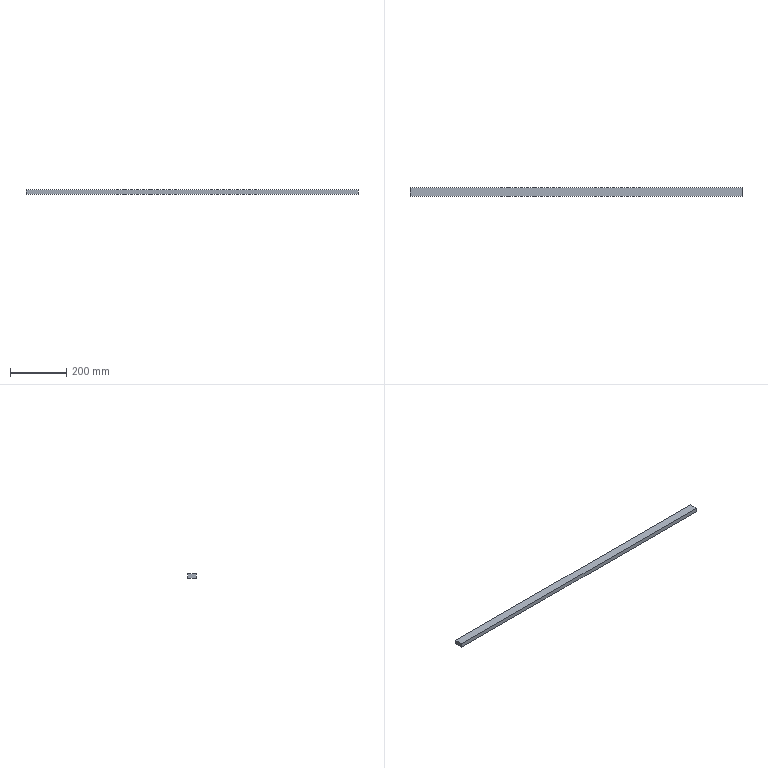Part | SolidWorks | features Extrusion 1 | 1 solid | 6 faces | box 1180 x 30 x 15 mm | volume 531000 mm3 | plane 6
STEP:
#1=CARTESIAN_POINT('',(590.,-15.,7.5));
#2=VERTEX_POINT('',#1);
#3=CARTESIAN_POINT('',(590.,-15.,-7.5));
#4=VERTEX_POINT('',#3);
#5=CARTESIAN_POINT('',(590.,-15.,7.5));
#6=DIRECTION('',(0.,0.,-1.));
#7=VECTOR('',#6,1000.);
#8=LINE('',#5,#7);
#9=EDGE_CURVE('',#2,#4,#8,.T.);
#10=ORIENTED_EDGE('',*,*,#9,.T.);
#11=CARTESIAN_POINT('',(590.,15.,-7.5));
#12=VERTEX_POINT('',#11);
#13=CARTESIAN_POINT('',(590.,15.,-7.5));
#14=DIRECTION('',(0.,-1.,0.));
#15=VECTOR('',#14,1000.);
#16=LINE('',#13,#15);
#17=EDGE_CURVE('',#12,#4,#16,.T.);
#18=ORIENTED_EDGE('',*,*,#17,.F.);
#19=CARTESIAN_POINT('',(590.,15.,7.5));
#20=VERTEX_POINT('',#19);
#21=CARTESIAN_POINT('',(590.,15.,7.5));
#22=DIRECTION('',(0.,0.,-1.));
#23=VECTOR('',#22,1000.);
#24=LINE('',#21,#23);
#25=EDGE_CURVE('',#20,#12,#24,.T.);
#26=ORIENTED_EDGE('',*,*,#25,.F.);
#27=CARTESIAN_POINT('',(590.,15.,7.5));
#28=DIRECTION('',(0.,-1.,0.));
#29=VECTOR('',#28,1000.);
#30=LINE('',#27,#29);
#31=EDGE_CURVE('',#20,#2,#30,.T.);
#32=ORIENTED_EDGE('',*,*,#31,.T.);
#33=EDGE_LOOP('',(#10,#18,#26,#32));
#34=FACE_OUTER_BOUND('',#33,.T.);
#35=CARTESIAN_POINT('',(590.,15.,7.5));
#36=DIRECTION('',(-1.,0.,0.));
#37=DIRECTION('',(0.,0.,1.));
#38=AXIS2_PLACEMENT_3D('',#35,#36,#37);
#39=PLANE('',#38);
#40=ADVANCED_FACE('',(#34),#39,.F.);
#41=CARTESIAN_POINT('',(-590.,-15.,-7.5));
#42=VERTEX_POINT('',#41);
#43=CARTESIAN_POINT('',(-590.,-15.,-7.5));
#44=DIRECTION('',(-1.,0.,0.));
#45=VECTOR('',#44,1000.);
#46=LINE('',#43,#45);
#47=EDGE_CURVE('',#4,#42,#46,.T.);
#48=ORIENTED_EDGE('',*,*,#47,.T.);
#49=CARTESIAN_POINT('',(-590.,15.,-7.5));
#50=VERTEX_POINT('',#49);
#51=CARTESIAN_POINT('',(-590.,15.,-7.5));
#52=DIRECTION('',(0.,-1.,0.));
#53=VECTOR('',#52,1000.);
#54=LINE('',#51,#53);
#55=EDGE_CURVE('',#50,#42,#54,.T.);
#56=ORIENTED_EDGE('',*,*,#55,.F.);
#57=CARTESIAN_POINT('',(-590.,15.,-7.5));
#58=DIRECTION('',(-1.,0.,0.));
#59=VECTOR('',#58,1000.);
#60=LINE('',#57,#59);
#61=EDGE_CURVE('',#12,#50,#60,.T.);
#62=ORIENTED_EDGE('',*,*,#61,.F.);
#63=ORIENTED_EDGE('',*,*,#17,.T.);
#64=EDGE_LOOP('',(#48,#56,#62,#63));
#65=FACE_OUTER_BOUND('',#64,.T.);
#66=CARTESIAN_POINT('',(-590.,15.,-7.5));
#67=DIRECTION('',(0.,0.,1.));
#68=DIRECTION('',(1.,0.,0.));
#69=AXIS2_PLACEMENT_3D('',#66,#67,#68);
#70=PLANE('',#69);
#71=ADVANCED_FACE('',(#65),#70,.F.);
#72=CARTESIAN_POINT('',(-590.,-15.,7.5));
#73=VERTEX_POINT('',#72);
#74=CARTESIAN_POINT('',(-590.,-15.,7.5));
#75=DIRECTION('',(0.,0.,1.));
#76=VECTOR('',#75,1000.);
#77=LINE('',#74,#76);
#78=EDGE_CURVE('',#42,#73,#77,.T.);
#79=ORIENTED_EDGE('',*,*,#78,.T.);
#80=CARTESIAN_POINT('',(-590.,15.,7.5));
#81=VERTEX_POINT('',#80);
#82=CARTESIAN_POINT('',(-590.,15.,7.5));
#83=DIRECTION('',(0.,-1.,0.));
#84=VECTOR('',#83,1000.);
#85=LINE('',#82,#84);
#86=EDGE_CURVE('',#81,#73,#85,.T.);
#87=ORIENTED_EDGE('',*,*,#86,.F.);
#88=CARTESIAN_POINT('',(-590.,15.,7.5));
#89=DIRECTION('',(0.,0.,1.));
#90=VECTOR('',#89,1000.);
#91=LINE('',#88,#90);
#92=EDGE_CURVE('',#50,#81,#91,.T.);
#93=ORIENTED_EDGE('',*,*,#92,.F.);
#94=ORIENTED_EDGE('',*,*,#55,.T.);
#95=EDGE_LOOP('',(#79,#87,#93,#94));
#96=FACE_OUTER_BOUND('',#95,.T.);
#97=CARTESIAN_POINT('',(-590.,15.,7.5));
#98=DIRECTION('',(1.,0.,0.));
#99=DIRECTION('',(0.,0.,-1.));
#100=AXIS2_PLACEMENT_3D('',#97,#98,#99);
#101=PLANE('',#100);
#102=ADVANCED_FACE('',(#96),#101,.F.);
#103=CARTESIAN_POINT('',(-590.,-15.,7.5));
#104=DIRECTION('',(1.,0.,0.));
#105=VECTOR('',#104,1000.);
#106=LINE('',#103,#105);
#107=EDGE_CURVE('',#73,#2,#106,.T.);
#108=ORIENTED_EDGE('',*,*,#107,.T.);
#109=ORIENTED_EDGE('',*,*,#31,.F.);
#110=CARTESIAN_POINT('',(-590.,15.,7.5));
#111=DIRECTION('',(1.,0.,0.));
#112=VECTOR('',#111,1000.);
#113=LINE('',#110,#112);
#114=EDGE_CURVE('',#81,#20,#113,.T.);
#115=ORIENTED_EDGE('',*,*,#114,.F.);
#116=ORIENTED_EDGE('',*,*,#86,.T.);
#117=EDGE_LOOP('',(#108,#109,#115,#116));
#118=FACE_OUTER_BOUND('',#117,.T.);
#119=CARTESIAN_POINT('',(-590.,15.,7.5));
#120=DIRECTION('',(0.,0.,-1.));
#121=DIRECTION('',(-1.,0.,0.));
#122=AXIS2_PLACEMENT_3D('',#119,#120,#121);
#123=PLANE('',#122);
#124=ADVANCED_FACE('',(#118),#123,.F.);
#125=ORIENTED_EDGE('',*,*,#25,.T.);
#126=ORIENTED_EDGE('',*,*,#61,.T.);
#127=ORIENTED_EDGE('',*,*,#92,.T.);
#128=ORIENTED_EDGE('',*,*,#114,.T.);
#129=EDGE_LOOP('',(#125,#126,#127,#128));
#130=FACE_OUTER_BOUND('',#129,.T.);
#131=CARTESIAN_POINT('',(0.,15.,0.));
#132=DIRECTION('',(0.,-1.,0.));
#133=DIRECTION('',(0.,0.,-1.));
#134=AXIS2_PLACEMENT_3D('',#131,#132,#133);
#135=PLANE('',#134);
#136=ADVANCED_FACE('',(#130),#135,.F.);
#137=ORIENTED_EDGE('',*,*,#9,.F.);
#138=ORIENTED_EDGE('',*,*,#107,.F.);
#139=ORIENTED_EDGE('',*,*,#78,.F.);
#140=ORIENTED_EDGE('',*,*,#47,.F.);
#141=EDGE_LOOP('',(#137,#138,#139,#140));
#142=FACE_OUTER_BOUND('',#141,.T.);
#143=CARTESIAN_POINT('',(0.,-15.,0.));
#144=DIRECTION('',(0.,-1.,0.));
#145=DIRECTION('',(0.,0.,-1.));
#146=AXIS2_PLACEMENT_3D('',#143,#144,#145);
#147=PLANE('',#146);
#148=ADVANCED_FACE('',(#142),#147,.T.);
#149=CLOSED_SHELL('',(#40,#71,#102,#124,#136,#148));
#150=MANIFOLD_SOLID_BREP('',#149);
#151=CARTESIAN_POINT('',(0.,0.,0.));
#152=DIRECTION('',(0.,0.,1.));
#153=DIRECTION('',(1.,0.,0.));
#154=AXIS2_PLACEMENT_3D('',#151,#152,#153);
#155=(LENGTH_UNIT()NAMED_UNIT(*)SI_UNIT(.MILLI.,.METRE.));
#156=UNCERTAINTY_MEASURE_WITH_UNIT(LENGTH_MEASURE(0.00001),#155,'','');
#157=(NAMED_UNIT(*)PLANE_ANGLE_UNIT()SI_UNIT($,.RADIAN.));
#158=(NAMED_UNIT(*)SI_UNIT($,.STERADIAN.)SOLID_ANGLE_UNIT());
#159=(GEOMETRIC_REPRESENTATION_CONTEXT(3)GLOBAL_UNCERTAINTY_ASSIGNED_CONTEXT((#156))GLOBAL_UNIT_ASSIGNED_CONTEXT((#155,#157,#158))REPRESENTATION_CONTEXT('',''));
#160=ADVANCED_BREP_SHAPE_REPRESENTATION('',(#150,#154),#159);